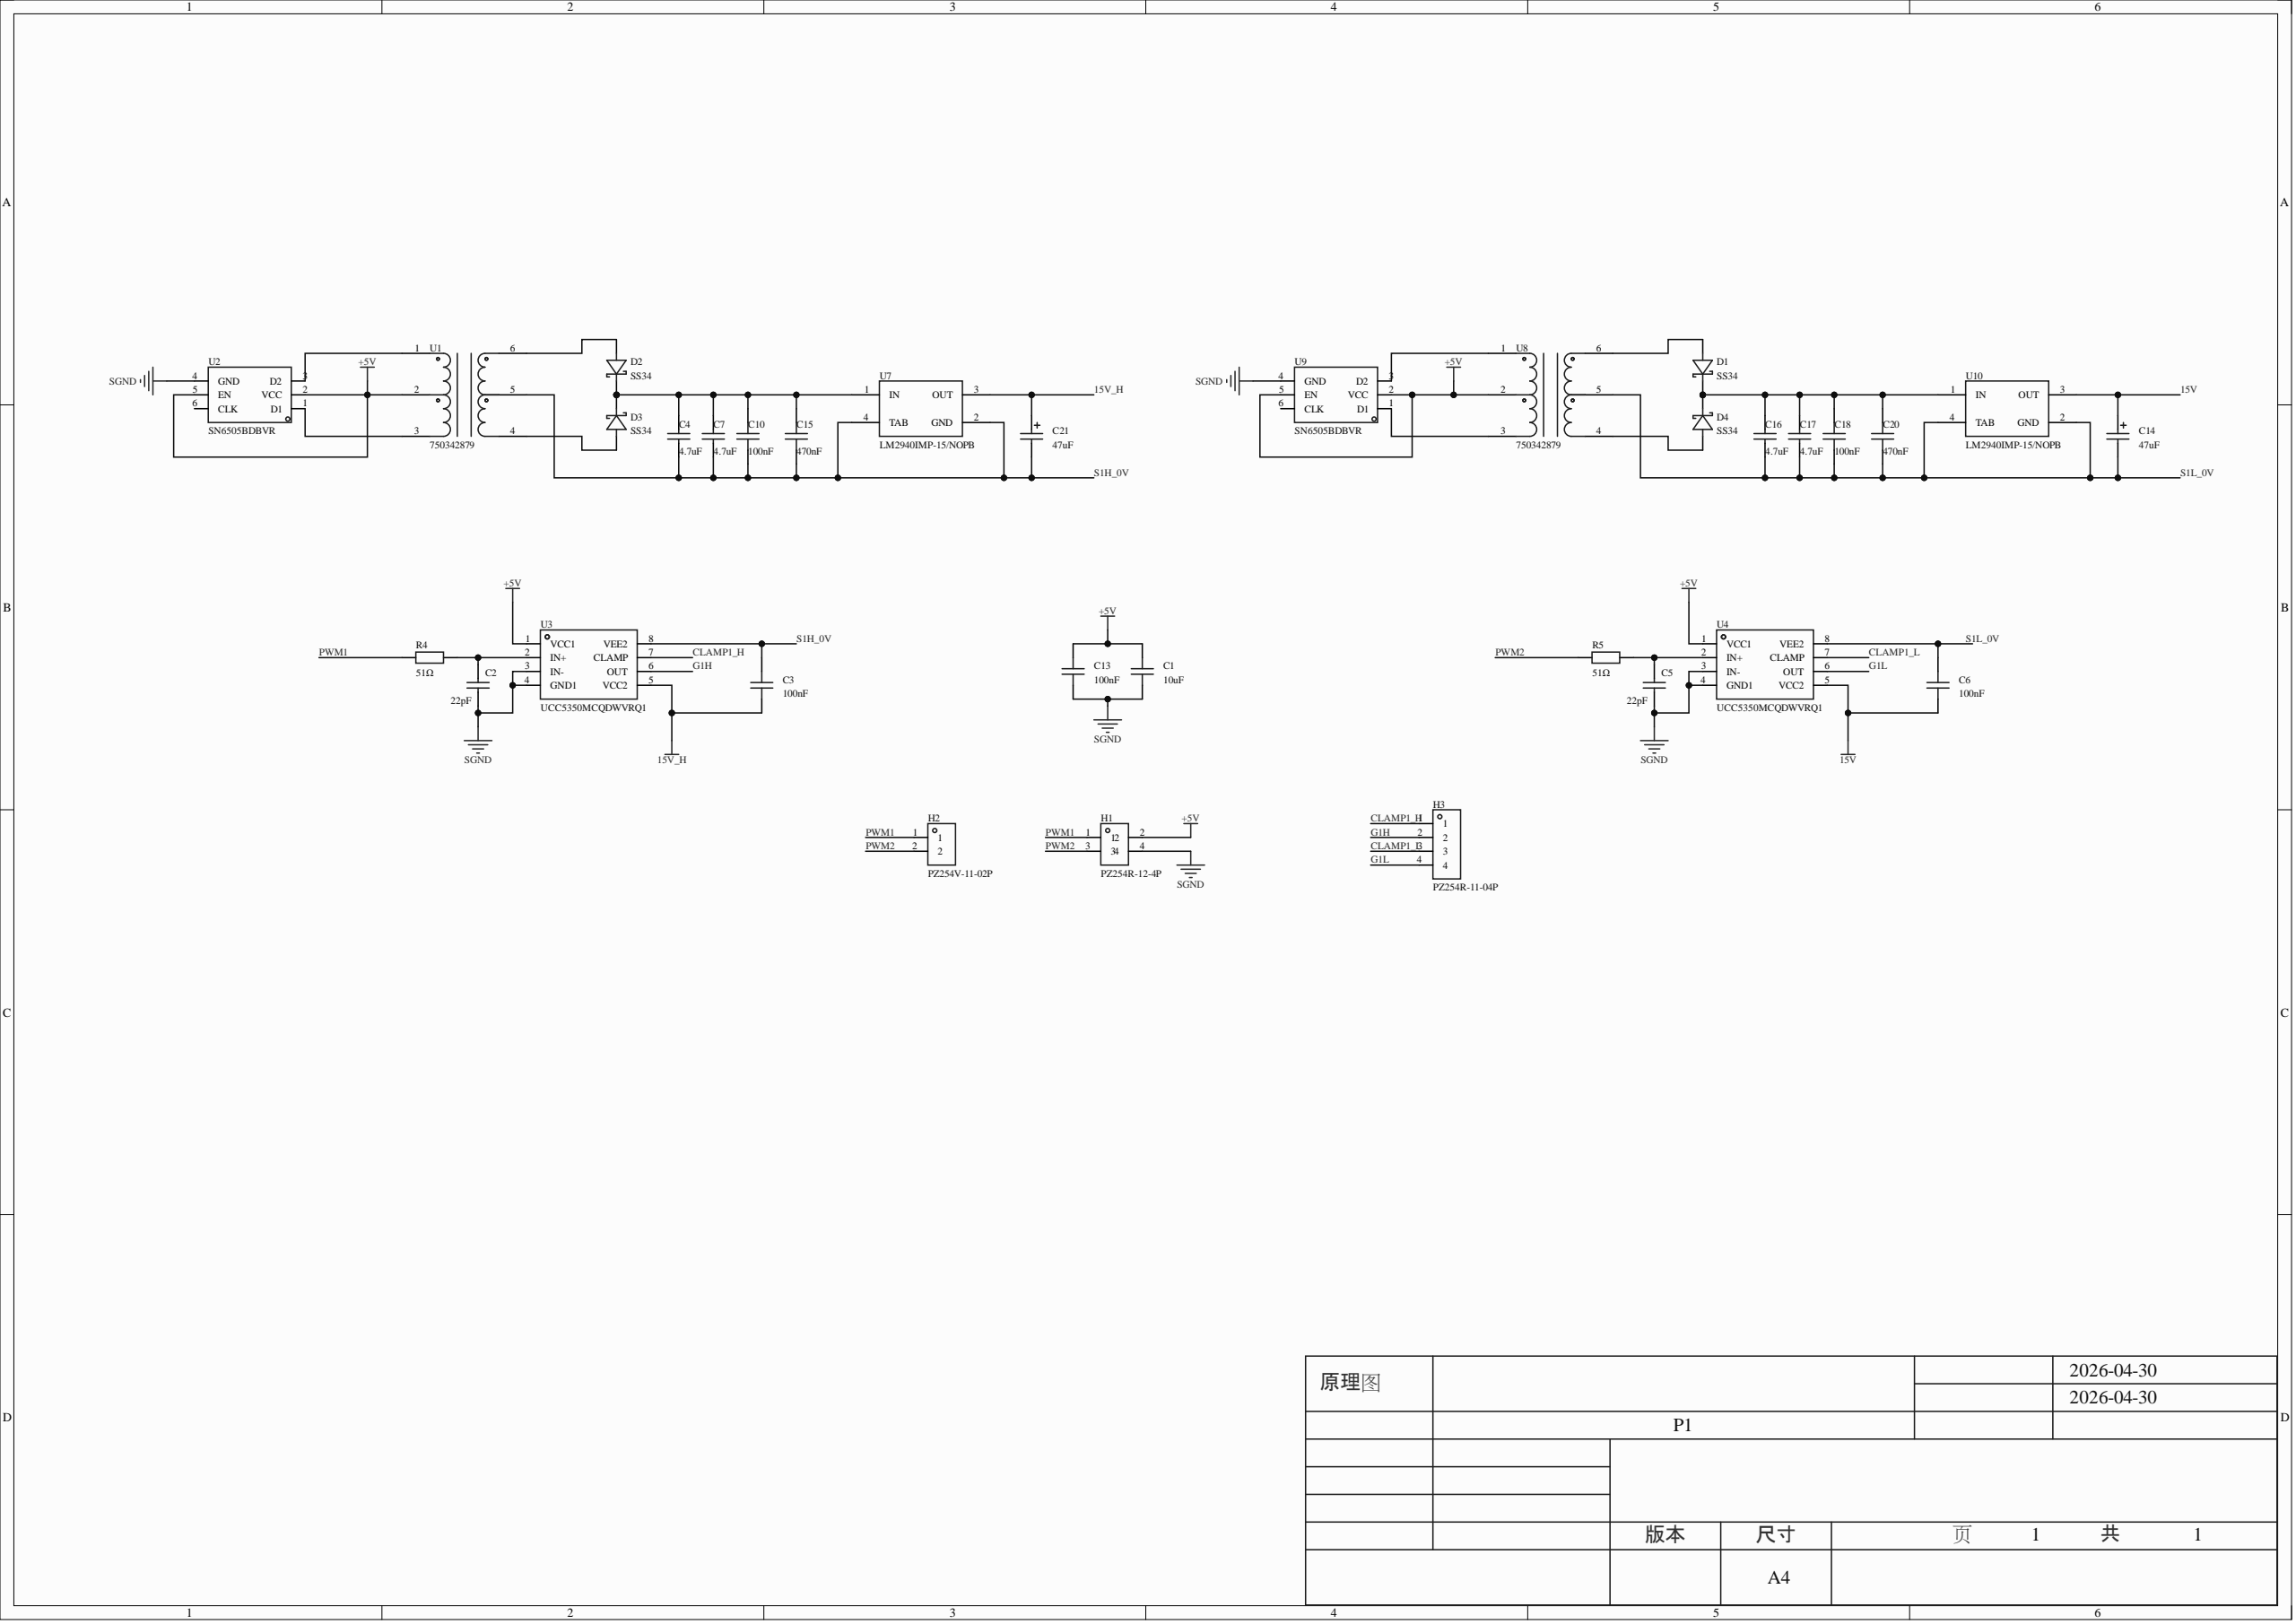Circuit board | Altium Designer | 33 parts | 24 nets
Bill of materials:
Comment,Description,Designator,Footprint,LibRef,Quantity
"10uF","容值:10uF;精度:±10%;额定电压:25V;温度系数:X5R;","C1","C0603","GRM188R61E106KA73D","1"
"22pF","容值:22pF;精度:±5%;额定电压:50V;温度系数:C0G;","C2, C5","C0402","0402CG220J500NT","2"
"100nF","容值:100nF;精度:±10%;额定电压:50V;温度系数:X7R;","C3, C6, C13","C0603","CGA0603X7R104K500JT","3"
"4.7uF","容值:4.7uF;精度:±10%;额定电压:50V;温度系数:X5R;","C4, C7, C16, C17","C0805","CL21A475KBQNNNE","4"
"100nF","容值:100nF;精度:±10%;额定电压:50V;温度系数:X7R;","C10, C18","CAP-SMD_L2.0-W1.25","FCC0805B104K500DT","2"
"47uF","","C14, C21","CAP-SMD_L7.3-W4.3-FD","T491X476K035AT","2"
"470nF","容值:470nF;精度:±10%;额定电压:50V;温度系数:X7R;","C15, C20","C0603","CC0603KRX7R9BB474","2"
"SS34","二极管配置:独立式;正向压降(Vf):550mV@3A;直流反向耐压(Vr):40V;整流电流:3A;","D1, D2, D3, D4","SMA_L4.3-W2.6-LS5.0-FD","SS34_C7420365","4"
"PZ254R-12-4P","插针结构:2x2P;间距:2.54mm;行距:2.54mm;圆针/方针:方针;安装方式:弯插;排数:双排;总PIN位数:4P;额定电流:-;额定电压:-;配合针长度:6mm;塑高:2.5mm;触头材质:黄铜;触头镀层:-;工作温度:-40℃~+105℃;颜色:黑色;","H1","HDR-TH_4P-P2.54-H-M-R2-C2-S2.54","PZ254R-12-4P","1"
"PZ254V-11-02P","插针结构:1x2P;间距:2.54mm;行距:-;圆针/方针:方针;安装方式:直插;排数:单排;总PIN位数:2P;额定电流:3A;额定电压:250V;配合针长度:6mm;塑高:2.5mm;端接针长度:3mm;触头材质:黄铜;触头镀层:-;工作温度:-40℃~+105℃;颜色:黑色;","H2","HDR-TH_2P-P2.54-V-M","PZ254V-11-02P","1"
"PZ254R-11-04P","插针结构:1x4P;间距:2.54mm;行距:-;圆针/方针:方针;安装方式:弯插;排数:单排;总PIN位数:4P;额定电流:3A;额定电压:250V;配合针长度:6mm;塑高:2.5mm;端接针长度:-;触头材质:黄铜;触头镀层:-;工作温度:-40℃~+105℃;颜色:黑色;","H3","HDR-TH_4P-P2.54-H-M-W10.4","PZ254R-11-04P","1"
"51Ω","","R4, R5","R0603","0603WAF510JT5E","2"
"750342879","","U1, U8","XFMR-SMD_6P-L9.1-W8.0-P3.05-LS13.0-TL","750342879","2"
"SN6505BDBVR","SN6505B 适用于隔离电源的低噪声、1A、420kHz 变压器驱动器","U2, U9","SOT-23-6_L2.9-W1.6-P0.95-LS2.8-BR","SN6505BDBVR","2"
"UCC5350MCQDWVRQ1","UCC5350-Q1 是一款单通道隔离式栅极驱动器，具有 5A 最小峰值拉电流和 5A 最小峰值灌电流，专为驱动 MOSFET、IGBT 和 SiC MOSFET 而设计。UCC5350-Q1 具有米勒钳位或分离输出选项。CLAMP 引脚除了可将晶体管栅极连接到输出端之外，还用于将栅极连接到内部 FET，以防止米勒电流造成假接通。借助分离输出选项，可以使用 OUTH 和 OUTL 引脚单独控制栅极电压的上升和下降时间。UCC5350-Q1 采用 4mm SOIC-8 (D) 或 8.5mm 宽体 SOIC","U3, U4","SOIC-8_L7.5-W5.9-P1.27-LS11.5-BL","UCC5350MCQDWVRQ1","2"
"LM2940IMP-15/NOPB","输出类型:固定;工作电压:26V;输出电压:15V;输出电流:1A;电源纹波抑制比(PSRR):-;输出极性:正极;","U7, U10","SOT-223-3_L6.5-W3.4-P2.30-LS7.0-BR","LM2940IMP-15/NOPB","2"
Netlist (Protel format):
[
C1
C0603
10uF



]
[
C2
C0402
22pF



]
[
C3
C0603
100nF



]
[
C4
C0805
4.7uF



]
[
C5
C0402
22pF



]
[
C6
C0603
100nF



]
[
C7
C0805
4.7uF



]
[
C10
CAP-SMD_L2.0-W1.25
100nF



]
[
C13
C0603
100nF



]
[
C14
CAP-SMD_L7.3-W4.3-FD
47uF



]
[
C15
C0603
470nF



]
[
C16
C0805
4.7uF



]
[
C17
C0805
4.7uF



]
[
C18
CAP-SMD_L2.0-W1.25
100nF



]
[
C20
C0603
470nF



]
[
C21
CAP-SMD_L7.3-W4.3-FD
47uF



]
[
D1
SMA_L4.3-W2.6-LS5.0-FD
SS34



]
[
D2
SMA_L4.3-W2.6-LS5.0-FD
SS34



]
[
D3
SMA_L4.3-W2.6-LS5.0-FD
SS34



]
[
D4
SMA_L4.3-W2.6-LS5.0-FD
SS34



]
[
H1
HDR-TH_4P-P2.54-H-M-R2-C2-S2.54
PZ254R-12-4P



]
[
H2
HDR-TH_2P-P2.54-V-M
PZ254V-11-02P



]
[
H3
HDR-TH_4P-P2.54-H-M-W10.4
PZ254R-11-04P



]
[
R4
R0603
51Ω



]
[
R5
R0603
51Ω



]
[
U1
XFMR-SMD_6P-L9.1-W8.0-P3.05-LS13.0-TL
750342879



]
[
U2
SOT-23-6_L2.9-W1.6-P0.95-LS2.8-BR
SN6505BDBVR



]
[
U3
SOIC-8_L7.5-W5.9-P1.27-LS11.5-BL
UCC5350MCQDWVRQ1



]
[
U4
SOIC-8_L7.5-W5.9-P1.27-LS11.5-BL
UCC5350MCQDWVRQ1



]
[
U7
SOT-223-3_L6.5-W3.4-P2.30-LS7.0-BR
LM2940IMP-15/NOPB



]
[
U8
XFMR-SMD_6P-L9.1-W8.0-P3.05-LS13.0-TL
750342879



]
[
U9
SOT-23-6_L2.9-W1.6-P0.95-LS2.8-BR
SN6505BDBVR



]
[
U10
SOT-223-3_L6.5-W3.4-P2.30-LS7.0-BR
LM2940IMP-15/NOPB



]
(
SGND
C1-2
C2-1
C5-1
C13-2
H1-4
U2-4
U3-3
U3-4
U4-3
U4-4
U9-4
)
(
S1L_0V
C6-1
C14-2
C16-1
C17-1
C18-1
C20-1
U4-8
U8-5
U10-2
U10-4
)
(
S1H_0V
C3-1
C4-1
C7-1
C10-1
C15-1
C21-2
U1-5
U3-8
U7-2
U7-4
)
(
PWM2
H1-3
H2-2
R5-1
)
(
PWM1
H1-1
H2-1
R4-1
)
(
NetU8_3
U8-3
U9-1
)
(
NetU8_1
U8-1
U9-3
)
(
NetU1_3
U1-3
U2-1
)
(
NetU1_1
U1-1
U2-3
)
(
NetD4_1
D4-1
U8-4
)
(
NetD3_1
D3-1
U1-4
)
(
NetD2_1
D2-1
U1-6
)
(
NetD1_1
D1-1
U8-6
)
(
NetC16_2
C16-2
C17-2
C18-2
C20-2
D1-2
D4-2
U10-1
)
(
NetC5_2
C5-2
R5-2
U4-2
)
(
NetC4_2
C4-2
C7-2
C10-2
C15-2
D2-2
D3-2
U7-1
)
(
NetC2_2
C2-2
R4-2
U3-2
)
(
G1L
H3-4
U4-6
)
(
G1H
H3-2
U3-6
)
(
CLAMP1_L
H3-3
U4-7
)
(
CLAMP1_H
H3-1
U3-7
)
(
+5V
C1-1
C13-1
H1-2
U1-2
U2-2
U2-5
U3-1
U4-1
U8-2
U9-2
U9-5
)
(
15V_H
C3-2
C21-1
U3-5
U7-3
)
(
15V
C6-2
C14-1
U4-5
U10-3
)